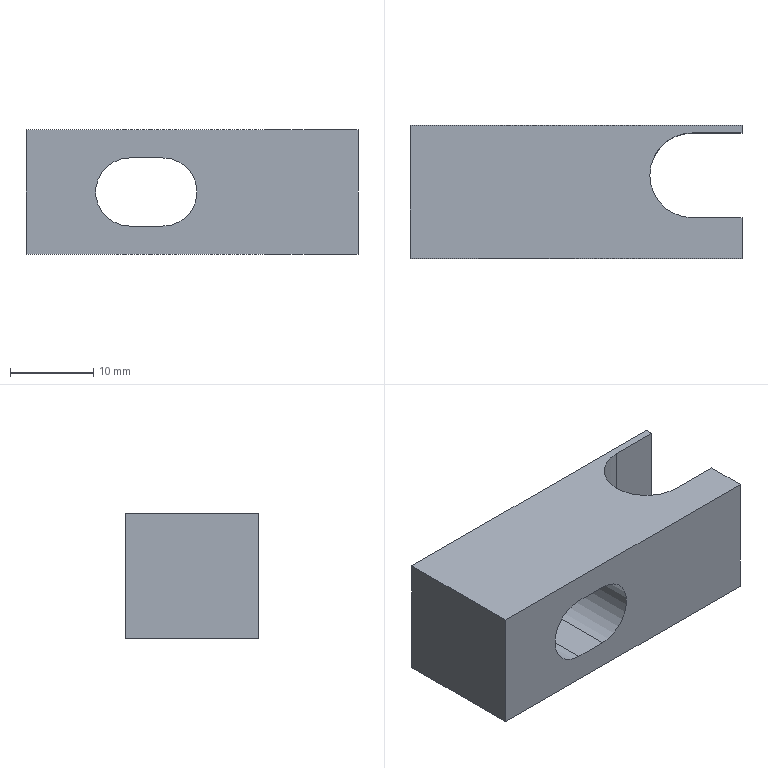Part | STEP file | 1 solid | 15 faces | box 40 x 16 x 15 mm | volume 6699 mm3 | plane 11 | cylinder 4 | commonest cylinder face diameters 8.2 x2 10.2 x2
STEP:
#1=CARTESIAN_POINT('',(0.,0.,0.));
#2=DIRECTION('',(0.,0.,1.));
#3=DIRECTION('',(1.,0.,0.));
#4=AXIS2_PLACEMENT_3D('',#1,#2,#3);
#5=CARTESIAN_POINT('',(9.9,2.077,15.));
#6=VERTEX_POINT('',#5);
#7=CARTESIAN_POINT('',(9.9,2.077,0.));
#8=VERTEX_POINT('',#7);
#9=CARTESIAN_POINT('',(9.9,2.077,15.));
#10=DIRECTION('',(0.,0.,-1.));
#11=VECTOR('',#10,1.);
#12=LINE('',#9,#11);
#13=CARTESIAN_POINT('',(9.9,-3.023,15.));
#14=DIRECTION('',(0.,0.,-1.));
#15=DIRECTION('',(-1.,0.,0.));
#16=AXIS2_PLACEMENT_3D('',#13,#14,#15);
#17=CYLINDRICAL_SURFACE('',#16,5.1);
#18=CARTESIAN_POINT('',(1.571,0.));
#19=DIRECTION('',(0.,1.));
#20=VECTOR('',#19,1.);
#21=LINE('',#18,#20);
#22=(GEOMETRIC_REPRESENTATION_CONTEXT(2)PARAMETRIC_REPRESENTATION_CONTEXT()REPRESENTATION_CONTEXT('',''));
#23=DEFINITIONAL_REPRESENTATION('',(#21),#22);
#24=PCURVE('',#17,#23);
#25=CARTESIAN_POINT('',(9.9,2.077,15.));
#26=DIRECTION('',(0.,1.,0.));
#27=DIRECTION('',(0.,0.,1.));
#28=AXIS2_PLACEMENT_3D('',#25,#26,#27);
#29=PLANE('',#28);
#30=CARTESIAN_POINT('',(0.,0.));
#31=DIRECTION('',(-1.,0.));
#32=VECTOR('',#31,1.);
#33=LINE('',#30,#32);
#34=(GEOMETRIC_REPRESENTATION_CONTEXT(2)PARAMETRIC_REPRESENTATION_CONTEXT()REPRESENTATION_CONTEXT('',''));
#35=DEFINITIONAL_REPRESENTATION('',(#33),#34);
#36=PCURVE('',#29,#35);
#37=SURFACE_CURVE('',#12,(#24,#36),.PCURVE_S1.);
#38=EDGE_CURVE('',#6,#8,#37,.T.);
#39=ORIENTED_EDGE('',*,*,#38,.T.);
#40=CARTESIAN_POINT('',(4.8,-3.023,0.));
#41=VERTEX_POINT('',#40);
#42=CARTESIAN_POINT('',(9.9,-3.023,0.));
#43=DIRECTION('',(0.,0.,-1.));
#44=DIRECTION('',(1.,0.,0.));
#45=AXIS2_PLACEMENT_3D('',#42,#43,#44);
#46=CIRCLE('',#45,5.1);
#47=CARTESIAN_POINT('',(-3.142,15.));
#48=DIRECTION('',(1.,0.));
#49=VECTOR('',#48,1.);
#50=LINE('',#47,#49);
#51=(GEOMETRIC_REPRESENTATION_CONTEXT(2)PARAMETRIC_REPRESENTATION_CONTEXT()REPRESENTATION_CONTEXT('',''));
#52=DEFINITIONAL_REPRESENTATION('',(#50),#51);
#53=PCURVE('',#17,#52);
#54=CARTESIAN_POINT('',(9.9,-3.023,0.));
#55=DIRECTION('',(0.,0.,1.));
#56=DIRECTION('',(1.,0.,0.));
#57=AXIS2_PLACEMENT_3D('',#54,#55,#56);
#58=PLANE('',#57);
#59=CARTESIAN_POINT('',(5.1,0.));
#60=CARTESIAN_POINT('',(5.1,-8.833));
#61=CARTESIAN_POINT('',(-2.55,-4.417));
#62=CARTESIAN_POINT('',(-10.2,0.));
#63=CARTESIAN_POINT('',(-2.55,4.417));
#64=CARTESIAN_POINT('',(5.1,8.833));
#65=CARTESIAN_POINT('',(5.1,0.));
#66=(BOUNDED_CURVE()B_SPLINE_CURVE(2,(#59,#60,#61,#62,#63,#64,#65),.UNSPECIFIED.,.T.,.F.)B_SPLINE_CURVE_WITH_KNOTS((1,2,2,2,2,1),(-2.094,0.,2.094,4.189,6.283,8.378),.UNSPECIFIED.)CURVE()GEOMETRIC_REPRESENTATION_ITEM()RATIONAL_B_SPLINE_CURVE((1.,0.5,1.,0.5,1.,0.5,1.))REPRESENTATION_ITEM(''));
#67=(GEOMETRIC_REPRESENTATION_CONTEXT(2)PARAMETRIC_REPRESENTATION_CONTEXT()REPRESENTATION_CONTEXT('',''));
#68=DEFINITIONAL_REPRESENTATION('',(#66),#67);
#69=PCURVE('',#58,#68);
#70=SURFACE_CURVE('',#46,(#53,#69),.PCURVE_S1.);
#71=EDGE_CURVE('',#41,#8,#70,.T.);
#72=ORIENTED_EDGE('',*,*,#71,.F.);
#73=CARTESIAN_POINT('',(4.8,-3.023,15.));
#74=VERTEX_POINT('',#73);
#75=CARTESIAN_POINT('',(4.8,-3.023,15.));
#76=DIRECTION('',(0.,0.,-1.));
#77=VECTOR('',#76,1.);
#78=LINE('',#75,#77);
#79=CARTESIAN_POINT('',(0.,0.));
#80=DIRECTION('',(0.,1.));
#81=VECTOR('',#80,1.);
#82=LINE('',#79,#81);
#83=(GEOMETRIC_REPRESENTATION_CONTEXT(2)PARAMETRIC_REPRESENTATION_CONTEXT()REPRESENTATION_CONTEXT('',''));
#84=DEFINITIONAL_REPRESENTATION('',(#82),#83);
#85=PCURVE('',#17,#84);
#86=CARTESIAN_POINT('',(9.9,-3.023,15.));
#87=DIRECTION('',(0.,0.,-1.));
#88=DIRECTION('',(-1.,0.,0.));
#89=AXIS2_PLACEMENT_3D('',#86,#87,#88);
#90=CYLINDRICAL_SURFACE('',#89,5.1);
#91=CARTESIAN_POINT('',(6.283,0.));
#92=DIRECTION('',(0.,1.));
#93=VECTOR('',#92,1.);
#94=LINE('',#91,#93);
#95=(GEOMETRIC_REPRESENTATION_CONTEXT(2)PARAMETRIC_REPRESENTATION_CONTEXT()REPRESENTATION_CONTEXT('',''));
#96=DEFINITIONAL_REPRESENTATION('',(#94),#95);
#97=PCURVE('',#90,#96);
#98=SURFACE_CURVE('',#78,(#85,#97),.PCURVE_S1.);
#99=EDGE_CURVE('',#74,#41,#98,.T.);
#100=ORIENTED_EDGE('',*,*,#99,.F.);
#101=CARTESIAN_POINT('',(9.9,-3.023,15.));
#102=DIRECTION('',(0.,0.,-1.));
#103=DIRECTION('',(1.,0.,0.));
#104=AXIS2_PLACEMENT_3D('',#101,#102,#103);
#105=CIRCLE('',#104,5.1);
#106=CARTESIAN_POINT('',(-3.142,0.));
#107=DIRECTION('',(1.,0.));
#108=VECTOR('',#107,1.);
#109=LINE('',#106,#108);
#110=(GEOMETRIC_REPRESENTATION_CONTEXT(2)PARAMETRIC_REPRESENTATION_CONTEXT()REPRESENTATION_CONTEXT('',''));
#111=DEFINITIONAL_REPRESENTATION('',(#109),#110);
#112=PCURVE('',#17,#111);
#113=CARTESIAN_POINT('',(9.9,-3.023,15.));
#114=DIRECTION('',(0.,0.,1.));
#115=DIRECTION('',(1.,0.,0.));
#116=AXIS2_PLACEMENT_3D('',#113,#114,#115);
#117=PLANE('',#116);
#118=CARTESIAN_POINT('',(5.1,0.));
#119=CARTESIAN_POINT('',(5.1,-8.833));
#120=CARTESIAN_POINT('',(-2.55,-4.417));
#121=CARTESIAN_POINT('',(-10.2,0.));
#122=CARTESIAN_POINT('',(-2.55,4.417));
#123=CARTESIAN_POINT('',(5.1,8.833));
#124=CARTESIAN_POINT('',(5.1,0.));
#125=(BOUNDED_CURVE()B_SPLINE_CURVE(2,(#118,#119,#120,#121,#122,#123,#124),.UNSPECIFIED.,.T.,.F.)B_SPLINE_CURVE_WITH_KNOTS((1,2,2,2,2,1),(-2.094,0.,2.094,4.189,6.283,8.378),.UNSPECIFIED.)CURVE()GEOMETRIC_REPRESENTATION_ITEM()RATIONAL_B_SPLINE_CURVE((1.,0.5,1.,0.5,1.,0.5,1.))REPRESENTATION_ITEM(''));
#126=(GEOMETRIC_REPRESENTATION_CONTEXT(2)PARAMETRIC_REPRESENTATION_CONTEXT()REPRESENTATION_CONTEXT('',''));
#127=DEFINITIONAL_REPRESENTATION('',(#125),#126);
#128=PCURVE('',#117,#127);
#129=SURFACE_CURVE('',#105,(#112,#128),.PCURVE_S1.);
#130=EDGE_CURVE('',#74,#6,#129,.T.);
#131=ORIENTED_EDGE('',*,*,#130,.T.);
#132=EDGE_LOOP('',(#39,#72,#100,#131));
#133=FACE_BOUND('',#132,.F.);
#134=ADVANCED_FACE('',(#133),#17,.F.);
#135=CARTESIAN_POINT('',(9.9,-8.123,0.));
#136=VERTEX_POINT('',#135);
#137=CARTESIAN_POINT('',(9.9,-3.023,0.));
#138=DIRECTION('',(0.,0.,-1.));
#139=DIRECTION('',(1.,0.,0.));
#140=AXIS2_PLACEMENT_3D('',#137,#138,#139);
#141=CIRCLE('',#140,5.1);
#142=CARTESIAN_POINT('',(3.142,15.));
#143=DIRECTION('',(1.,0.));
#144=VECTOR('',#143,1.);
#145=LINE('',#142,#144);
#146=(GEOMETRIC_REPRESENTATION_CONTEXT(2)PARAMETRIC_REPRESENTATION_CONTEXT()REPRESENTATION_CONTEXT('',''));
#147=DEFINITIONAL_REPRESENTATION('',(#145),#146);
#148=PCURVE('',#90,#147);
#149=CARTESIAN_POINT('',(5.1,0.));
#150=CARTESIAN_POINT('',(5.1,-8.833));
#151=CARTESIAN_POINT('',(-2.55,-4.417));
#152=CARTESIAN_POINT('',(-10.2,0.));
#153=CARTESIAN_POINT('',(-2.55,4.417));
#154=CARTESIAN_POINT('',(5.1,8.833));
#155=CARTESIAN_POINT('',(5.1,0.));
#156=(BOUNDED_CURVE()B_SPLINE_CURVE(2,(#149,#150,#151,#152,#153,#154,#155),.UNSPECIFIED.,.T.,.F.)B_SPLINE_CURVE_WITH_KNOTS((1,2,2,2,2,1),(-2.094,0.,2.094,4.189,6.283,8.378),.UNSPECIFIED.)CURVE()GEOMETRIC_REPRESENTATION_ITEM()RATIONAL_B_SPLINE_CURVE((1.,0.5,1.,0.5,1.,0.5,1.))REPRESENTATION_ITEM(''));
#157=(GEOMETRIC_REPRESENTATION_CONTEXT(2)PARAMETRIC_REPRESENTATION_CONTEXT()REPRESENTATION_CONTEXT('',''));
#158=DEFINITIONAL_REPRESENTATION('',(#156),#157);
#159=PCURVE('',#58,#158);
#160=SURFACE_CURVE('',#141,(#148,#159),.PCURVE_S1.);
#161=EDGE_CURVE('',#136,#41,#160,.T.);
#162=ORIENTED_EDGE('',*,*,#161,.F.);
#163=CARTESIAN_POINT('',(9.9,-8.123,15.));
#164=VERTEX_POINT('',#163);
#165=CARTESIAN_POINT('',(9.9,-8.123,15.));
#166=DIRECTION('',(0.,0.,-1.));
#167=VECTOR('',#166,1.);
#168=LINE('',#165,#167);
#169=CARTESIAN_POINT('',(4.712,0.));
#170=DIRECTION('',(0.,1.));
#171=VECTOR('',#170,1.);
#172=LINE('',#169,#171);
#173=(GEOMETRIC_REPRESENTATION_CONTEXT(2)PARAMETRIC_REPRESENTATION_CONTEXT()REPRESENTATION_CONTEXT('',''));
#174=DEFINITIONAL_REPRESENTATION('',(#172),#173);
#175=PCURVE('',#90,#174);
#176=CARTESIAN_POINT('',(9.9,-8.123,15.));
#177=DIRECTION('',(0.,-1.,0.));
#178=DIRECTION('',(0.,0.,-1.));
#179=AXIS2_PLACEMENT_3D('',#176,#177,#178);
#180=PLANE('',#179);
#181=CARTESIAN_POINT('',(0.,0.));
#182=DIRECTION('',(1.,0.));
#183=VECTOR('',#182,1.);
#184=LINE('',#181,#183);
#185=(GEOMETRIC_REPRESENTATION_CONTEXT(2)PARAMETRIC_REPRESENTATION_CONTEXT()REPRESENTATION_CONTEXT('',''));
#186=DEFINITIONAL_REPRESENTATION('',(#184),#185);
#187=PCURVE('',#180,#186);
#188=SURFACE_CURVE('',#168,(#175,#187),.PCURVE_S1.);
#189=EDGE_CURVE('',#164,#136,#188,.T.);
#190=ORIENTED_EDGE('',*,*,#189,.F.);
#191=CARTESIAN_POINT('',(9.9,-3.023,15.));
#192=DIRECTION('',(0.,0.,-1.));
#193=DIRECTION('',(1.,0.,0.));
#194=AXIS2_PLACEMENT_3D('',#191,#192,#193);
#195=CIRCLE('',#194,5.1);
#196=CARTESIAN_POINT('',(3.142,0.));
#197=DIRECTION('',(1.,0.));
#198=VECTOR('',#197,1.);
#199=LINE('',#196,#198);
#200=(GEOMETRIC_REPRESENTATION_CONTEXT(2)PARAMETRIC_REPRESENTATION_CONTEXT()REPRESENTATION_CONTEXT('',''));
#201=DEFINITIONAL_REPRESENTATION('',(#199),#200);
#202=PCURVE('',#90,#201);
#203=CARTESIAN_POINT('',(5.1,0.));
#204=CARTESIAN_POINT('',(5.1,-8.833));
#205=CARTESIAN_POINT('',(-2.55,-4.417));
#206=CARTESIAN_POINT('',(-10.2,0.));
#207=CARTESIAN_POINT('',(-2.55,4.417));
#208=CARTESIAN_POINT('',(5.1,8.833));
#209=CARTESIAN_POINT('',(5.1,0.));
#210=(BOUNDED_CURVE()B_SPLINE_CURVE(2,(#203,#204,#205,#206,#207,#208,#209),.UNSPECIFIED.,.T.,.F.)B_SPLINE_CURVE_WITH_KNOTS((1,2,2,2,2,1),(-2.094,0.,2.094,4.189,6.283,8.378),.UNSPECIFIED.)CURVE()GEOMETRIC_REPRESENTATION_ITEM()RATIONAL_B_SPLINE_CURVE((1.,0.5,1.,0.5,1.,0.5,1.))REPRESENTATION_ITEM(''));
#211=(GEOMETRIC_REPRESENTATION_CONTEXT(2)PARAMETRIC_REPRESENTATION_CONTEXT()REPRESENTATION_CONTEXT('',''));
#212=DEFINITIONAL_REPRESENTATION('',(#210),#211);
#213=PCURVE('',#117,#212);
#214=SURFACE_CURVE('',#195,(#202,#213),.PCURVE_S1.);
#215=EDGE_CURVE('',#164,#74,#214,.T.);
#216=ORIENTED_EDGE('',*,*,#215,.T.);
#217=ORIENTED_EDGE('',*,*,#99,.T.);
#218=EDGE_LOOP('',(#162,#190,#216,#217));
#219=FACE_BOUND('',#218,.F.);
#220=ADVANCED_FACE('',(#219),#90,.F.);
#221=CARTESIAN_POINT('',(15.9,2.077,0.));
#222=VERTEX_POINT('',#221);
#223=CARTESIAN_POINT('',(9.9,2.077,0.));
#224=DIRECTION('',(1.,0.,0.));
#225=VECTOR('',#224,1.);
#226=LINE('',#223,#225);
#227=CARTESIAN_POINT('',(-15.,0.));
#228=DIRECTION('',(0.,1.));
#229=VECTOR('',#228,1.);
#230=LINE('',#227,#229);
#231=(GEOMETRIC_REPRESENTATION_CONTEXT(2)PARAMETRIC_REPRESENTATION_CONTEXT()REPRESENTATION_CONTEXT('',''));
#232=DEFINITIONAL_REPRESENTATION('',(#230),#231);
#233=PCURVE('',#29,#232);
#234=CARTESIAN_POINT('',(0.,5.1));
#235=DIRECTION('',(1.,0.));
#236=VECTOR('',#235,1.);
#237=LINE('',#234,#236);
#238=(GEOMETRIC_REPRESENTATION_CONTEXT(2)PARAMETRIC_REPRESENTATION_CONTEXT()REPRESENTATION_CONTEXT('',''));
#239=DEFINITIONAL_REPRESENTATION('',(#237),#238);
#240=PCURVE('',#58,#239);
#241=SURFACE_CURVE('',#226,(#233,#240),.PCURVE_S1.);
#242=EDGE_CURVE('',#8,#222,#241,.T.);
#243=ORIENTED_EDGE('',*,*,#242,.T.);
#244=CARTESIAN_POINT('',(15.9,2.077,15.));
#245=VERTEX_POINT('',#244);
#246=CARTESIAN_POINT('',(15.9,2.077,15.));
#247=DIRECTION('',(0.,0.,-1.));
#248=VECTOR('',#247,1.);
#249=LINE('',#246,#248);
#250=CARTESIAN_POINT('',(0.,6.));
#251=DIRECTION('',(-1.,0.));
#252=VECTOR('',#251,1.);
#253=LINE('',#250,#252);
#254=(GEOMETRIC_REPRESENTATION_CONTEXT(2)PARAMETRIC_REPRESENTATION_CONTEXT()REPRESENTATION_CONTEXT('',''));
#255=DEFINITIONAL_REPRESENTATION('',(#253),#254);
#256=PCURVE('',#29,#255);
#257=CARTESIAN_POINT('',(15.9,2.977,15.));
#258=DIRECTION('',(-1.,0.,0.));
#259=DIRECTION('',(0.,0.,1.));
#260=AXIS2_PLACEMENT_3D('',#257,#258,#259);
#261=PLANE('',#260);
#262=CARTESIAN_POINT('',(0.,-0.9));
#263=DIRECTION('',(-1.,0.));
#264=VECTOR('',#263,1.);
#265=LINE('',#262,#264);
#266=(GEOMETRIC_REPRESENTATION_CONTEXT(2)PARAMETRIC_REPRESENTATION_CONTEXT()REPRESENTATION_CONTEXT('',''));
#267=DEFINITIONAL_REPRESENTATION('',(#265),#266);
#268=PCURVE('',#261,#267);
#269=SURFACE_CURVE('',#249,(#256,#268),.PCURVE_S1.);
#270=EDGE_CURVE('',#245,#222,#269,.T.);
#271=ORIENTED_EDGE('',*,*,#270,.F.);
#272=CARTESIAN_POINT('',(9.9,2.077,15.));
#273=DIRECTION('',(1.,0.,0.));
#274=VECTOR('',#273,1.);
#275=LINE('',#272,#274);
#276=CARTESIAN_POINT('',(0.,0.));
#277=DIRECTION('',(0.,1.));
#278=VECTOR('',#277,1.);
#279=LINE('',#276,#278);
#280=(GEOMETRIC_REPRESENTATION_CONTEXT(2)PARAMETRIC_REPRESENTATION_CONTEXT()REPRESENTATION_CONTEXT('',''));
#281=DEFINITIONAL_REPRESENTATION('',(#279),#280);
#282=PCURVE('',#29,#281);
#283=CARTESIAN_POINT('',(0.,5.1));
#284=DIRECTION('',(1.,0.));
#285=VECTOR('',#284,1.);
#286=LINE('',#283,#285);
#287=(GEOMETRIC_REPRESENTATION_CONTEXT(2)PARAMETRIC_REPRESENTATION_CONTEXT()REPRESENTATION_CONTEXT('',''));
#288=DEFINITIONAL_REPRESENTATION('',(#286),#287);
#289=PCURVE('',#117,#288);
#290=SURFACE_CURVE('',#275,(#282,#289),.PCURVE_S1.);
#291=EDGE_CURVE('',#6,#245,#290,.T.);
#292=ORIENTED_EDGE('',*,*,#291,.F.);
#293=ORIENTED_EDGE('',*,*,#38,.T.);
#294=EDGE_LOOP('',(#243,#271,#292,#293));
#295=FACE_BOUND('',#294,.T.);
#296=ADVANCED_FACE('',(#295),#29,.F.);
#297=CARTESIAN_POINT('',(15.9,2.977,0.));
#298=VERTEX_POINT('',#297);
#299=CARTESIAN_POINT('',(15.9,2.977,0.));
#300=DIRECTION('',(0.,1.,0.));
#301=VECTOR('',#300,1.);
#302=LINE('',#299,#301);
#303=CARTESIAN_POINT('',(-15.,0.));
#304=DIRECTION('',(0.,1.));
#305=VECTOR('',#304,1.);
#306=LINE('',#303,#305);
#307=(GEOMETRIC_REPRESENTATION_CONTEXT(2)PARAMETRIC_REPRESENTATION_CONTEXT()REPRESENTATION_CONTEXT('',''));
#308=DEFINITIONAL_REPRESENTATION('',(#306),#307);
#309=PCURVE('',#261,#308);
#310=CARTESIAN_POINT('',(6.,6.));
#311=DIRECTION('',(0.,1.));
#312=VECTOR('',#311,1.);
#313=LINE('',#310,#312);
#314=(GEOMETRIC_REPRESENTATION_CONTEXT(2)PARAMETRIC_REPRESENTATION_CONTEXT()REPRESENTATION_CONTEXT('',''));
#315=DEFINITIONAL_REPRESENTATION('',(#313),#314);
#316=PCURVE('',#58,#315);
#317=SURFACE_CURVE('',#302,(#309,#316),.PCURVE_S1.);
#318=EDGE_CURVE('',#222,#298,#317,.T.);
#319=ORIENTED_EDGE('',*,*,#318,.T.);
#320=CARTESIAN_POINT('',(15.9,2.977,15.));
#321=VERTEX_POINT('',#320);
#322=CARTESIAN_POINT('',(15.9,2.977,15.));
#323=DIRECTION('',(0.,0.,-1.));
#324=VECTOR('',#323,1.);
#325=LINE('',#322,#324);
#326=CARTESIAN_POINT('',(0.,0.));
#327=DIRECTION('',(-1.,0.));
#328=VECTOR('',#327,1.);
#329=LINE('',#326,#328);
#330=(GEOMETRIC_REPRESENTATION_CONTEXT(2)PARAMETRIC_REPRESENTATION_CONTEXT()REPRESENTATION_CONTEXT('',''));
#331=DEFINITIONAL_REPRESENTATION('',(#329),#330);
#332=PCURVE('',#261,#331);
#333=CARTESIAN_POINT('',(-24.1,2.977,15.));
#334=DIRECTION('',(0.,-1.,0.));
#335=DIRECTION('',(1.,0.,0.));
#336=AXIS2_PLACEMENT_3D('',#333,#334,#335);
#337=PLANE('',#336);
#338=CARTESIAN_POINT('',(40.,0.));
#339=DIRECTION('',(0.,-1.));
#340=VECTOR('',#339,1.);
#341=LINE('',#338,#340);
#342=(GEOMETRIC_REPRESENTATION_CONTEXT(2)PARAMETRIC_REPRESENTATION_CONTEXT()REPRESENTATION_CONTEXT('',''));
#343=DEFINITIONAL_REPRESENTATION('',(#341),#342);
#344=PCURVE('',#337,#343);
#345=SURFACE_CURVE('',#325,(#332,#344),.PCURVE_S1.);
#346=EDGE_CURVE('',#321,#298,#345,.T.);
#347=ORIENTED_EDGE('',*,*,#346,.F.);
#348=CARTESIAN_POINT('',(15.9,2.977,15.));
#349=DIRECTION('',(0.,1.,0.));
#350=VECTOR('',#349,1.);
#351=LINE('',#348,#350);
#352=CARTESIAN_POINT('',(0.,0.));
#353=DIRECTION('',(0.,1.));
#354=VECTOR('',#353,1.);
#355=LINE('',#352,#354);
#356=(GEOMETRIC_REPRESENTATION_CONTEXT(2)PARAMETRIC_REPRESENTATION_CONTEXT()REPRESENTATION_CONTEXT('',''));
#357=DEFINITIONAL_REPRESENTATION('',(#355),#356);
#358=PCURVE('',#261,#357);
#359=CARTESIAN_POINT('',(6.,6.));
#360=DIRECTION('',(0.,1.));
#361=VECTOR('',#360,1.);
#362=LINE('',#359,#361);
#363=(GEOMETRIC_REPRESENTATION_CONTEXT(2)PARAMETRIC_REPRESENTATION_CONTEXT()REPRESENTATION_CONTEXT('',''));
#364=DEFINITIONAL_REPRESENTATION('',(#362),#363);
#365=PCURVE('',#117,#364);
#366=SURFACE_CURVE('',#351,(#358,#365),.PCURVE_S1.);
#367=EDGE_CURVE('',#245,#321,#366,.T.);
#368=ORIENTED_EDGE('',*,*,#367,.F.);
#369=ORIENTED_EDGE('',*,*,#270,.T.);
#370=EDGE_LOOP('',(#319,#347,#368,#369));
#371=FACE_BOUND('',#370,.T.);
#372=ADVANCED_FACE('',(#371),#261,.F.);
#373=CARTESIAN_POINT('',(-11.6,2.977,3.4));
#374=VERTEX_POINT('',#373);
#375=CARTESIAN_POINT('',(-7.6,2.977,3.4));
#376=VERTEX_POINT('',#375);
#377=CARTESIAN_POINT('',(-7.6,2.977,3.4));
#378=DIRECTION('',(1.,0.,0.));
#379=VECTOR('',#378,1.);
#380=LINE('',#377,#379);
#381=CARTESIAN_POINT('',(16.5,-11.6));
#382=DIRECTION('',(1.,0.));
#383=VECTOR('',#382,1.);
#384=LINE('',#381,#383);
#385=(GEOMETRIC_REPRESENTATION_CONTEXT(2)PARAMETRIC_REPRESENTATION_CONTEXT()REPRESENTATION_CONTEXT('',''));
#386=DEFINITIONAL_REPRESENTATION('',(#384),#385);
#387=PCURVE('',#337,#386);
#388=CARTESIAN_POINT('',(-7.6,2.977,3.4));
#389=DIRECTION('',(0.,0.,-1.));
#390=DIRECTION('',(-1.,0.,0.));
#391=AXIS2_PLACEMENT_3D('',#388,#389,#390);
#392=PLANE('',#391);
#393=CARTESIAN_POINT('',(0.,0.));
#394=DIRECTION('',(-1.,0.));
#395=VECTOR('',#394,1.);
#396=LINE('',#393,#395);
#397=(GEOMETRIC_REPRESENTATION_CONTEXT(2)PARAMETRIC_REPRESENTATION_CONTEXT()REPRESENTATION_CONTEXT('',''));
#398=DEFINITIONAL_REPRESENTATION('',(#396),#397);
#399=PCURVE('',#392,#398);
#400=SURFACE_CURVE('',#380,(#387,#399),.PCURVE_S1.);
#401=EDGE_CURVE('',#374,#376,#400,.T.);
#402=ORIENTED_EDGE('',*,*,#401,.T.);
#403=CARTESIAN_POINT('',(-7.6,2.977,11.6));
#404=VERTEX_POINT('',#403);
#405=CARTESIAN_POINT('',(-7.6,2.977,7.5));
#406=DIRECTION('',(0.,-1.,0.));
#407=DIRECTION('',(0.,0.,-1.));
#408=AXIS2_PLACEMENT_3D('',#405,#406,#407);
#409=CIRCLE('',#408,4.1);
#410=CARTESIAN_POINT('',(16.5,-7.5));
#411=DIRECTION('',(0.,-1.));
#412=AXIS2_PLACEMENT_2D('',#410,#411);
#413=CIRCLE('',#412,4.1);
#414=(GEOMETRIC_REPRESENTATION_CONTEXT(2)PARAMETRIC_REPRESENTATION_CONTEXT()REPRESENTATION_CONTEXT('',''));
#415=DEFINITIONAL_REPRESENTATION('',(#413),#414);
#416=PCURVE('',#337,#415);
#417=CARTESIAN_POINT('',(-7.6,2.977,7.5));
#418=DIRECTION('',(0.,-1.,0.));
#419=DIRECTION('',(0.,0.,-1.));
#420=AXIS2_PLACEMENT_3D('',#417,#418,#419);
#421=CYLINDRICAL_SURFACE('',#420,4.1);
#422=CARTESIAN_POINT('',(0.,0.));
#423=DIRECTION('',(1.,0.));
#424=VECTOR('',#423,1.);
#425=LINE('',#422,#424);
#426=(GEOMETRIC_REPRESENTATION_CONTEXT(2)PARAMETRIC_REPRESENTATION_CONTEXT()REPRESENTATION_CONTEXT('',''));
#427=DEFINITIONAL_REPRESENTATION('',(#425),#426);
#428=PCURVE('',#421,#427);
#429=SURFACE_CURVE('',#409,(#416,#428),.PCURVE_S1.);
#430=EDGE_CURVE('',#376,#404,#429,.T.);
#431=ORIENTED_EDGE('',*,*,#430,.T.);
#432=CARTESIAN_POINT('',(-11.6,2.977,11.6));
#433=VERTEX_POINT('',#432);
#434=CARTESIAN_POINT('',(-7.6,2.977,11.6));
#435=DIRECTION('',(-1.,0.,0.));
#436=VECTOR('',#435,1.);
#437=LINE('',#434,#436);
#438=CARTESIAN_POINT('',(16.5,-3.4));
#439=DIRECTION('',(-1.,0.));
#440=VECTOR('',#439,1.);
#441=LINE('',#438,#440);
#442=(GEOMETRIC_REPRESENTATION_CONTEXT(2)PARAMETRIC_REPRESENTATION_CONTEXT()REPRESENTATION_CONTEXT('',''));
#443=DEFINITIONAL_REPRESENTATION('',(#441),#442);
#444=PCURVE('',#337,#443);
#445=CARTESIAN_POINT('',(-7.6,2.977,11.6));
#446=DIRECTION('',(0.,0.,1.));
#447=DIRECTION('',(1.,0.,0.));
#448=AXIS2_PLACEMENT_3D('',#445,#446,#447);
#449=PLANE('',#448);
#450=CARTESIAN_POINT('',(0.,0.));
#451=DIRECTION('',(-1.,0.));
#452=VECTOR('',#451,1.);
#453=LINE('',#450,#452);
#454=(GEOMETRIC_REPRESENTATION_CONTEXT(2)PARAMETRIC_REPRESENTATION_CONTEXT()REPRESENTATION_CONTEXT('',''));
#455=DEFINITIONAL_REPRESENTATION('',(#453),#454);
#456=PCURVE('',#449,#455);
#457=SURFACE_CURVE('',#437,(#444,#456),.PCURVE_S1.);
#458=EDGE_CURVE('',#404,#433,#457,.T.);
#459=ORIENTED_EDGE('',*,*,#458,.T.);
#460=CARTESIAN_POINT('',(-11.6,2.977,7.5));
#461=DIRECTION('',(0.,-1.,0.));
#462=DIRECTION('',(0.,0.,-1.));
#463=AXIS2_PLACEMENT_3D('',#460,#461,#462);
#464=CIRCLE('',#463,4.1);
#465=CARTESIAN_POINT('',(12.5,-7.5));
#466=DIRECTION('',(0.,-1.));
#467=AXIS2_PLACEMENT_2D('',#465,#466);
#468=CIRCLE('',#467,4.1);
#469=(GEOMETRIC_REPRESENTATION_CONTEXT(2)PARAMETRIC_REPRESENTATION_CONTEXT()REPRESENTATION_CONTEXT('',''));
#470=DEFINITIONAL_REPRESENTATION('',(#468),#469);
#471=PCURVE('',#337,#470);
#472=CARTESIAN_POINT('',(-11.6,2.977,7.5));
#473=DIRECTION('',(0.,-1.,0.));
#474=DIRECTION('',(0.,0.,-1.));
#475=AXIS2_PLACEMENT_3D('',#472,#473,#474);
#476=CYLINDRICAL_SURFACE('',#475,4.1);
#477=CARTESIAN_POINT('',(0.,0.));
#478=DIRECTION('',(1.,0.));
#479=VECTOR('',#478,1.);
#480=LINE('',#477,#479);
#481=(GEOMETRIC_REPRESENTATION_CONTEXT(2)PARAMETRIC_REPRESENTATION_CONTEXT()REPRESENTATION_CONTEXT('',''));
#482=DEFINITIONAL_REPRESENTATION('',(#480),#481);
#483=PCURVE('',#476,#482);
#484=SURFACE_CURVE('',#464,(#471,#483),.PCURVE_S1.);
#485=EDGE_CURVE('',#433,#374,#484,.T.);
#486=ORIENTED_EDGE('',*,*,#485,.T.);
#487=EDGE_LOOP('',(#402,#431,#459,#486));
#488=FACE_BOUND('',#487,.T.);
#489=CARTESIAN_POINT('',(-24.1,2.977,0.));
#490=VERTEX_POINT('',#489);
#491=CARTESIAN_POINT('',(-24.1,2.977,0.));
#492=DIRECTION('',(-1.,0.,0.));
#493=VECTOR('',#492,1.);
#494=LINE('',#491,#493);
#495=CARTESIAN_POINT('',(0.,-15.));
#496=DIRECTION('',(-1.,0.));
#497=VECTOR('',#496,1.);
#498=LINE('',#495,#497);
#499=(GEOMETRIC_REPRESENTATION_CONTEXT(2)PARAMETRIC_REPRESENTATION_CONTEXT()REPRESENTATION_CONTEXT('',''));
#500=DEFINITIONAL_REPRESENTATION('',(#498),#499);
#501=PCURVE('',#337,#500);
#502=CARTESIAN_POINT('',(-34.,6.));
#503=DIRECTION('',(-1.,0.));
#504=VECTOR('',#503,1.);
#505=LINE('',#502,#504);
#506=(GEOMETRIC_REPRESENTATION_CONTEXT(2)PARAMETRIC_REPRESENTATION_CONTEXT()REPRESENTATION_CONTEXT('',''));
#507=DEFINITIONAL_REPRESENTATION('',(#505),#506);
#508=PCURVE('',#58,#507);
#509=SURFACE_CURVE('',#494,(#501,#508),.PCURVE_S1.);
#510=EDGE_CURVE('',#298,#490,#509,.T.);
#511=ORIENTED_EDGE('',*,*,#510,.T.);
#512=CARTESIAN_POINT('',(-24.1,2.977,15.));
#513=VERTEX_POINT('',#512);
#514=CARTESIAN_POINT('',(-24.1,2.977,15.));
#515=DIRECTION('',(0.,0.,-1.));
#516=VECTOR('',#515,1.);
#517=LINE('',#514,#516);
#518=CARTESIAN_POINT('',(0.,0.));
#519=DIRECTION('',(0.,-1.));
#520=VECTOR('',#519,1.);
#521=LINE('',#518,#520);
#522=(GEOMETRIC_REPRESENTATION_CONTEXT(2)PARAMETRIC_REPRESENTATION_CONTEXT()REPRESENTATION_CONTEXT('',''));
#523=DEFINITIONAL_REPRESENTATION('',(#521),#522);
#524=PCURVE('',#337,#523);
#525=CARTESIAN_POINT('',(-24.1,2.977,15.));
#526=DIRECTION('',(1.,0.,0.));
#527=DIRECTION('',(0.,0.,-1.));
#528=AXIS2_PLACEMENT_3D('',#525,#526,#527);
#529=PLANE('',#528);
#530=CARTESIAN_POINT('',(0.,0.));
#531=DIRECTION('',(1.,0.));
#532=VECTOR('',#531,1.);
#533=LINE('',#530,#532);
#534=(GEOMETRIC_REPRESENTATION_CONTEXT(2)PARAMETRIC_REPRESENTATION_CONTEXT()REPRESENTATION_CONTEXT('',''));
#535=DEFINITIONAL_REPRESENTATION('',(#533),#534);
#536=PCURVE('',#529,#535);
#537=SURFACE_CURVE('',#517,(#524,#536),.PCURVE_S1.);
#538=EDGE_CURVE('',#513,#490,#537,.T.);
#539=ORIENTED_EDGE('',*,*,#538,.F.);
#540=CARTESIAN_POINT('',(-24.1,2.977,15.));
#541=DIRECTION('',(-1.,0.,0.));
#542=VECTOR('',#541,1.);
#543=LINE('',#540,#542);
#544=CARTESIAN_POINT('',(0.,0.));
#545=DIRECTION('',(-1.,0.));
#546=VECTOR('',#545,1.);
#547=LINE('',#544,#546);
#548=(GEOMETRIC_REPRESENTATION_CONTEXT(2)PARAMETRIC_REPRESENTATION_CONTEXT()REPRESENTATION_CONTEXT('',''));
#549=DEFINITIONAL_REPRESENTATION('',(#547),#548);
#550=PCURVE('',#337,#549);
#551=CARTESIAN_POINT('',(-34.,6.));
#552=DIRECTION('',(-1.,0.));
#553=VECTOR('',#552,1.);
#554=LINE('',#551,#553);
#555=(GEOMETRIC_REPRESENTATION_CONTEXT(2)PARAMETRIC_REPRESENTATION_CONTEXT()REPRESENTATION_CONTEXT('',''));
#556=DEFINITIONAL_REPRESENTATION('',(#554),#555);
#557=PCURVE('',#117,#556);
#558=SURFACE_CURVE('',#543,(#550,#557),.PCURVE_S1.);
#559=EDGE_CURVE('',#321,#513,#558,.T.);
#560=ORIENTED_EDGE('',*,*,#559,.F.);
#561=ORIENTED_EDGE('',*,*,#346,.T.);
#562=EDGE_LOOP('',(#511,#539,#560,#561));
#563=FACE_BOUND('',#562,.T.);
#564=ADVANCED_FACE('',(#488,#563),#337,.F.);
#565=CARTESIAN_POINT('',(-24.1,-13.023,0.));
#566=VERTEX_POINT('',#565);
#567=CARTESIAN_POINT('',(-24.1,2.977,0.));
#568=DIRECTION('',(0.,-1.,0.));
#569=VECTOR('',#568,1.);
#570=LINE('',#567,#569);
#571=CARTESIAN_POINT('',(15.,0.));
#572=DIRECTION('',(0.,-1.));
#573=VECTOR('',#572,1.);
#574=LINE('',#571,#573);
#575=(GEOMETRIC_REPRESENTATION_CONTEXT(2)PARAMETRIC_REPRESENTATION_CONTEXT()REPRESENTATION_CONTEXT('',''));
#576=DEFINITIONAL_REPRESENTATION('',(#574),#575);
#577=PCURVE('',#529,#576);
#578=CARTESIAN_POINT('',(-34.,6.));
#579=DIRECTION('',(0.,-1.));
#580=VECTOR('',#579,1.);
#581=LINE('',#578,#580);
#582=(GEOMETRIC_REPRESENTATION_CONTEXT(2)PARAMETRIC_REPRESENTATION_CONTEXT()REPRESENTATION_CONTEXT('',''));
#583=DEFINITIONAL_REPRESENTATION('',(#581),#582);
#584=PCURVE('',#58,#583);
#585=SURFACE_CURVE('',#570,(#577,#584),.PCURVE_S1.);
#586=EDGE_CURVE('',#490,#566,#585,.T.);
#587=ORIENTED_EDGE('',*,*,#586,.T.);
#588=CARTESIAN_POINT('',(-24.1,-13.023,15.));
#589=VERTEX_POINT('',#588);
#590=CARTESIAN_POINT('',(-24.1,-13.023,15.));
#591=DIRECTION('',(0.,0.,-1.));
#592=VECTOR('',#591,1.);
#593=LINE('',#590,#592);
#594=CARTESIAN_POINT('',(0.,-16.));
#595=DIRECTION('',(1.,0.));
#596=VECTOR('',#595,1.);
#597=LINE('',#594,#596);
#598=(GEOMETRIC_REPRESENTATION_CONTEXT(2)PARAMETRIC_REPRESENTATION_CONTEXT()REPRESENTATION_CONTEXT('',''));
#599=DEFINITIONAL_REPRESENTATION('',(#597),#598);
#600=PCURVE('',#529,#599);
#601=CARTESIAN_POINT('',(-24.1,-13.023,15.));
#602=DIRECTION('',(0.,1.,0.));
#603=DIRECTION('',(0.,0.,1.));
#604=AXIS2_PLACEMENT_3D('',#601,#602,#603);
#605=PLANE('',#604);
#606=CARTESIAN_POINT('',(0.,0.));
#607=DIRECTION('',(-1.,0.));
#608=VECTOR('',#607,1.);
#609=LINE('',#606,#608);
#610=(GEOMETRIC_REPRESENTATION_CONTEXT(2)PARAMETRIC_REPRESENTATION_CONTEXT()REPRESENTATION_CONTEXT('',''));
#611=DEFINITIONAL_REPRESENTATION('',(#609),#610);
#612=PCURVE('',#605,#611);
#613=SURFACE_CURVE('',#593,(#600,#612),.PCURVE_S1.);
#614=EDGE_CURVE('',#589,#566,#613,.T.);
#615=ORIENTED_EDGE('',*,*,#614,.F.);
#616=CARTESIAN_POINT('',(-24.1,2.977,15.));
#617=DIRECTION('',(0.,-1.,0.));
#618=VECTOR('',#617,1.);
#619=LINE('',#616,#618);
#620=CARTESIAN_POINT('',(0.,0.));
#621=DIRECTION('',(0.,-1.));
#622=VECTOR('',#621,1.);
#623=LINE('',#620,#622);
#624=(GEOMETRIC_REPRESENTATION_CONTEXT(2)PARAMETRIC_REPRESENTATION_CONTEXT()REPRESENTATION_CONTEXT('',''));
#625=DEFINITIONAL_REPRESENTATION('',(#623),#624);
#626=PCURVE('',#529,#625);
#627=CARTESIAN_POINT('',(-34.,6.));
#628=DIRECTION('',(0.,-1.));
#629=VECTOR('',#628,1.);
#630=LINE('',#627,#629);
#631=(GEOMETRIC_REPRESENTATION_CONTEXT(2)PARAMETRIC_REPRESENTATION_CONTEXT()REPRESENTATION_CONTEXT('',''));
#632=DEFINITIONAL_REPRESENTATION('',(#630),#631);
#633=PCURVE('',#117,#632);
#634=SURFACE_CURVE('',#619,(#626,#633),.PCURVE_S1.);
#635=EDGE_CURVE('',#513,#589,#634,.T.);
#636=ORIENTED_EDGE('',*,*,#635,.F.);
#637=ORIENTED_EDGE('',*,*,#538,.T.);
#638=EDGE_LOOP('',(#587,#615,#636,#637));
#639=FACE_BOUND('',#638,.T.);
#640=ADVANCED_FACE('',(#639),#529,.F.);
#641=CARTESIAN_POINT('',(-7.6,-13.023,11.6));
#642=VERTEX_POINT('',#641);
#643=CARTESIAN_POINT('',(-11.6,-13.023,11.6));
#644=VERTEX_POINT('',#643);
#645=CARTESIAN_POINT('',(-7.6,-13.023,11.6));
#646=DIRECTION('',(-1.,0.,0.));
#647=VECTOR('',#646,1.);
#648=LINE('',#645,#647);
#649=CARTESIAN_POINT('',(-3.4,16.5));
#650=DIRECTION('',(0.,-1.));
#651=VECTOR('',#650,1.);
#652=LINE('',#649,#651);
#653=(GEOMETRIC_REPRESENTATION_CONTEXT(2)PARAMETRIC_REPRESENTATION_CONTEXT()REPRESENTATION_CONTEXT('',''));
#654=DEFINITIONAL_REPRESENTATION('',(#652),#653);
#655=PCURVE('',#605,#654);
#656=CARTESIAN_POINT('',(0.,-16.));
#657=DIRECTION('',(-1.,0.));
#658=VECTOR('',#657,1.);
#659=LINE('',#656,#658);
#660=(GEOMETRIC_REPRESENTATION_CONTEXT(2)PARAMETRIC_REPRESENTATION_CONTEXT()REPRESENTATION_CONTEXT('',''));
#661=DEFINITIONAL_REPRESENTATION('',(#659),#660);
#662=PCURVE('',#449,#661);
#663=SURFACE_CURVE('',#648,(#655,#662),.PCURVE_S1.);
#664=EDGE_CURVE('',#642,#644,#663,.T.);
#665=ORIENTED_EDGE('',*,*,#664,.F.);
#666=CARTESIAN_POINT('',(-7.6,-13.023,3.4));
#667=VERTEX_POINT('',#666);
#668=CARTESIAN_POINT('',(-7.6,-13.023,7.5));
#669=DIRECTION('',(0.,-1.,0.));
#670=DIRECTION('',(0.,0.,-1.));
#671=AXIS2_PLACEMENT_3D('',#668,#669,#670);
#672=CIRCLE('',#671,4.1);
#673=CARTESIAN_POINT('',(-11.6,16.5));
#674=CARTESIAN_POINT('',(-11.6,23.601));
#675=CARTESIAN_POINT('',(-5.45,20.051));
#676=CARTESIAN_POINT('',(0.7,16.5));
#677=CARTESIAN_POINT('',(-5.45,12.949));
#678=CARTESIAN_POINT('',(-11.6,9.399));
#679=CARTESIAN_POINT('',(-11.6,16.5));
#680=(BOUNDED_CURVE()B_SPLINE_CURVE(2,(#673,#674,#675,#676,#677,#678,#679),.UNSPECIFIED.,.T.,.F.)B_SPLINE_CURVE_WITH_KNOTS((1,2,2,2,2,1),(-2.094,0.,2.094,4.189,6.283,8.378),.UNSPECIFIED.)CURVE()GEOMETRIC_REPRESENTATION_ITEM()RATIONAL_B_SPLINE_CURVE((1.,0.5,1.,0.5,1.,0.5,1.))REPRESENTATION_ITEM(''));
#681=(GEOMETRIC_REPRESENTATION_CONTEXT(2)PARAMETRIC_REPRESENTATION_CONTEXT()REPRESENTATION_CONTEXT('',''));
#682=DEFINITIONAL_REPRESENTATION('',(#680),#681);
#683=PCURVE('',#605,#682);
#684=CARTESIAN_POINT('',(0.,16.));
#685=DIRECTION('',(1.,0.));
#686=VECTOR('',#685,1.);
#687=LINE('',#684,#686);
#688=(GEOMETRIC_REPRESENTATION_CONTEXT(2)PARAMETRIC_REPRESENTATION_CONTEXT()REPRESENTATION_CONTEXT('',''));
#689=DEFINITIONAL_REPRESENTATION('',(#687),#688);
#690=PCURVE('',#421,#689);
#691=SURFACE_CURVE('',#672,(#683,#690),.PCURVE_S1.);
#692=EDGE_CURVE('',#667,#642,#691,.T.);
#693=ORIENTED_EDGE('',*,*,#692,.F.);
#694=CARTESIAN_POINT('',(-11.6,-13.023,3.4));
#695=VERTEX_POINT('',#694);
#696=CARTESIAN_POINT('',(-7.6,-13.023,3.4));
#697=DIRECTION('',(1.,0.,0.));
#698=VECTOR('',#697,1.);
#699=LINE('',#696,#698);
#700=CARTESIAN_POINT('',(-11.6,16.5));
#701=DIRECTION('',(0.,1.));
#702=VECTOR('',#701,1.);
#703=LINE('',#700,#702);
#704=(GEOMETRIC_REPRESENTATION_CONTEXT(2)PARAMETRIC_REPRESENTATION_CONTEXT()REPRESENTATION_CONTEXT('',''));
#705=DEFINITIONAL_REPRESENTATION('',(#703),#704);
#706=PCURVE('',#605,#705);
#707=CARTESIAN_POINT('',(0.,-16.));
#708=DIRECTION('',(-1.,0.));
#709=VECTOR('',#708,1.);
#710=LINE('',#707,#709);
#711=(GEOMETRIC_REPRESENTATION_CONTEXT(2)PARAMETRIC_REPRESENTATION_CONTEXT()REPRESENTATION_CONTEXT('',''));
#712=DEFINITIONAL_REPRESENTATION('',(#710),#711);
#713=PCURVE('',#392,#712);
#714=SURFACE_CURVE('',#699,(#706,#713),.PCURVE_S1.);
#715=EDGE_CURVE('',#695,#667,#714,.T.);
#716=ORIENTED_EDGE('',*,*,#715,.F.);
#717=CARTESIAN_POINT('',(-11.6,-13.023,7.5));
#718=DIRECTION('',(0.,-1.,0.));
#719=DIRECTION('',(0.,0.,-1.));
#720=AXIS2_PLACEMENT_3D('',#717,#718,#719);
#721=CIRCLE('',#720,4.1);
#722=CARTESIAN_POINT('',(-11.6,12.5));
#723=CARTESIAN_POINT('',(-11.6,19.601));
#724=CARTESIAN_POINT('',(-5.45,16.051));
#725=CARTESIAN_POINT('',(0.7,12.5));
#726=CARTESIAN_POINT('',(-5.45,8.949));
#727=CARTESIAN_POINT('',(-11.6,5.399));
#728=CARTESIAN_POINT('',(-11.6,12.5));
#729=(BOUNDED_CURVE()B_SPLINE_CURVE(2,(#722,#723,#724,#725,#726,#727,#728),.UNSPECIFIED.,.T.,.F.)B_SPLINE_CURVE_WITH_KNOTS((1,2,2,2,2,1),(-2.094,0.,2.094,4.189,6.283,8.378),.UNSPECIFIED.)CURVE()GEOMETRIC_REPRESENTATION_ITEM()RATIONAL_B_SPLINE_CURVE((1.,0.5,1.,0.5,1.,0.5,1.))REPRESENTATION_ITEM(''));
#730=(GEOMETRIC_REPRESENTATION_CONTEXT(2)PARAMETRIC_REPRESENTATION_CONTEXT()REPRESENTATION_CONTEXT('',''));
#731=DEFINITIONAL_REPRESENTATION('',(#729),#730);
#732=PCURVE('',#605,#731);
#733=CARTESIAN_POINT('',(0.,16.));
#734=DIRECTION('',(1.,0.));
#735=VECTOR('',#734,1.);
#736=LINE('',#733,#735);
#737=(GEOMETRIC_REPRESENTATION_CONTEXT(2)PARAMETRIC_REPRESENTATION_CONTEXT()REPRESENTATION_CONTEXT('',''));
#738=DEFINITIONAL_REPRESENTATION('',(#736),#737);
#739=PCURVE('',#476,#738);
#740=SURFACE_CURVE('',#721,(#732,#739),.PCURVE_S1.);
#741=EDGE_CURVE('',#644,#695,#740,.T.);
#742=ORIENTED_EDGE('',*,*,#741,.F.);
#743=EDGE_LOOP('',(#665,#693,#716,#742));
#744=FACE_BOUND('',#743,.T.);
#745=CARTESIAN_POINT('',(15.9,-13.023,0.));
#746=VERTEX_POINT('',#745);
#747=CARTESIAN_POINT('',(-24.1,-13.023,0.));
#748=DIRECTION('',(1.,0.,0.));
#749=VECTOR('',#748,1.);
#750=LINE('',#747,#749);
#751=CARTESIAN_POINT('',(-15.,0.));
#752=DIRECTION('',(0.,1.));
#753=VECTOR('',#752,1.);
#754=LINE('',#751,#753);
#755=(GEOMETRIC_REPRESENTATION_CONTEXT(2)PARAMETRIC_REPRESENTATION_CONTEXT()REPRESENTATION_CONTEXT('',''));
#756=DEFINITIONAL_REPRESENTATION('',(#754),#755);
#757=PCURVE('',#605,#756);
#758=CARTESIAN_POINT('',(-34.,-10.));
#759=DIRECTION('',(1.,0.));
#760=VECTOR('',#759,1.);
#761=LINE('',#758,#760);
#762=(GEOMETRIC_REPRESENTATION_CONTEXT(2)PARAMETRIC_REPRESENTATION_CONTEXT()REPRESENTATION_CONTEXT('',''));
#763=DEFINITIONAL_REPRESENTATION('',(#761),#762);
#764=PCURVE('',#58,#763);
#765=SURFACE_CURVE('',#750,(#757,#764),.PCURVE_S1.);
#766=EDGE_CURVE('',#566,#746,#765,.T.);
#767=ORIENTED_EDGE('',*,*,#766,.T.);
#768=CARTESIAN_POINT('',(15.9,-13.023,15.));
#769=VERTEX_POINT('',#768);
#770=CARTESIAN_POINT('',(15.9,-13.023,15.));
#771=DIRECTION('',(0.,0.,-1.));
#772=VECTOR('',#771,1.);
#773=LINE('',#770,#772);
#774=CARTESIAN_POINT('',(0.,40.));
#775=DIRECTION('',(-1.,0.));
#776=VECTOR('',#775,1.);
#777=LINE('',#774,#776);
#778=(GEOMETRIC_REPRESENTATION_CONTEXT(2)PARAMETRIC_REPRESENTATION_CONTEXT()REPRESENTATION_CONTEXT('',''));
#779=DEFINITIONAL_REPRESENTATION('',(#777),#778);
#780=PCURVE('',#605,#779);
#781=CARTESIAN_POINT('',(15.9,-8.123,15.));
#782=DIRECTION('',(-1.,0.,0.));
#783=DIRECTION('',(0.,0.,1.));
#784=AXIS2_PLACEMENT_3D('',#781,#782,#783);
#785=PLANE('',#784);
#786=CARTESIAN_POINT('',(0.,-4.9));
#787=DIRECTION('',(-1.,0.));
#788=VECTOR('',#787,1.);
#789=LINE('',#786,#788);
#790=(GEOMETRIC_REPRESENTATION_CONTEXT(2)PARAMETRIC_REPRESENTATION_CONTEXT()REPRESENTATION_CONTEXT('',''));
#791=DEFINITIONAL_REPRESENTATION('',(#789),#790);
#792=PCURVE('',#785,#791);
#793=SURFACE_CURVE('',#773,(#780,#792),.PCURVE_S1.);
#794=EDGE_CURVE('',#769,#746,#793,.T.);
#795=ORIENTED_EDGE('',*,*,#794,.F.);
#796=CARTESIAN_POINT('',(-24.1,-13.023,15.));
#797=DIRECTION('',(1.,0.,0.));
#798=VECTOR('',#797,1.);
#799=LINE('',#796,#798);
#800=CARTESIAN_POINT('',(0.,0.));
#801=DIRECTION('',(0.,1.));
#802=VECTOR('',#801,1.);
#803=LINE('',#800,#802);
#804=(GEOMETRIC_REPRESENTATION_CONTEXT(2)PARAMETRIC_REPRESENTATION_CONTEXT()REPRESENTATION_CONTEXT('',''));
#805=DEFINITIONAL_REPRESENTATION('',(#803),#804);
#806=PCURVE('',#605,#805);
#807=CARTESIAN_POINT('',(-34.,-10.));
#808=DIRECTION('',(1.,0.));
#809=VECTOR('',#808,1.);
#810=LINE('',#807,#809);
#811=(GEOMETRIC_REPRESENTATION_CONTEXT(2)PARAMETRIC_REPRESENTATION_CONTEXT()REPRESENTATION_CONTEXT('',''));
#812=DEFINITIONAL_REPRESENTATION('',(#810),#811);
#813=PCURVE('',#117,#812);
#814=SURFACE_CURVE('',#799,(#806,#813),.PCURVE_S1.);
#815=EDGE_CURVE('',#589,#769,#814,.T.);
#816=ORIENTED_EDGE('',*,*,#815,.F.);
#817=ORIENTED_EDGE('',*,*,#614,.T.);
#818=EDGE_LOOP('',(#767,#795,#816,#817));
#819=FACE_BOUND('',#818,.T.);
#820=ADVANCED_FACE('',(#744,#819),#605,.F.);
#821=CARTESIAN_POINT('',(15.9,-8.123,0.));
#822=VERTEX_POINT('',#821);
#823=CARTESIAN_POINT('',(15.9,-8.123,0.));
#824=DIRECTION('',(0.,1.,0.));
#825=VECTOR('',#824,1.);
#826=LINE('',#823,#825);
#827=CARTESIAN_POINT('',(-15.,0.));
#828=DIRECTION('',(0.,1.));
#829=VECTOR('',#828,1.);
#830=LINE('',#827,#829);
#831=(GEOMETRIC_REPRESENTATION_CONTEXT(2)PARAMETRIC_REPRESENTATION_CONTEXT()REPRESENTATION_CONTEXT('',''));
#832=DEFINITIONAL_REPRESENTATION('',(#830),#831);
#833=PCURVE('',#785,#832);
#834=CARTESIAN_POINT('',(6.,-5.1));
#835=DIRECTION('',(0.,1.));
#836=VECTOR('',#835,1.);
#837=LINE('',#834,#836);
#838=(GEOMETRIC_REPRESENTATION_CONTEXT(2)PARAMETRIC_REPRESENTATION_CONTEXT()REPRESENTATION_CONTEXT('',''));
#839=DEFINITIONAL_REPRESENTATION('',(#837),#838);
#840=PCURVE('',#58,#839);
#841=SURFACE_CURVE('',#826,(#833,#840),.PCURVE_S1.);
#842=EDGE_CURVE('',#746,#822,#841,.T.);
#843=ORIENTED_EDGE('',*,*,#842,.T.);
#844=CARTESIAN_POINT('',(15.9,-8.123,15.));
#845=VERTEX_POINT('',#844);
#846=CARTESIAN_POINT('',(15.9,-8.123,15.));
#847=DIRECTION('',(0.,0.,-1.));
#848=VECTOR('',#847,1.);
#849=LINE('',#846,#848);
#850=CARTESIAN_POINT('',(0.,0.));
#851=DIRECTION('',(-1.,0.));
#852=VECTOR('',#851,1.);
#853=LINE('',#850,#852);
#854=(GEOMETRIC_REPRESENTATION_CONTEXT(2)PARAMETRIC_REPRESENTATION_CONTEXT()REPRESENTATION_CONTEXT('',''));
#855=DEFINITIONAL_REPRESENTATION('',(#853),#854);
#856=PCURVE('',#785,#855);
#857=CARTESIAN_POINT('',(0.,6.));
#858=DIRECTION('',(1.,0.));
#859=VECTOR('',#858,1.);
#860=LINE('',#857,#859);
#861=(GEOMETRIC_REPRESENTATION_CONTEXT(2)PARAMETRIC_REPRESENTATION_CONTEXT()REPRESENTATION_CONTEXT('',''));
#862=DEFINITIONAL_REPRESENTATION('',(#860),#861);
#863=PCURVE('',#180,#862);
#864=SURFACE_CURVE('',#849,(#856,#863),.PCURVE_S1.);
#865=EDGE_CURVE('',#845,#822,#864,.T.);
#866=ORIENTED_EDGE('',*,*,#865,.F.);
#867=CARTESIAN_POINT('',(15.9,-8.123,15.));
#868=DIRECTION('',(0.,1.,0.));
#869=VECTOR('',#868,1.);
#870=LINE('',#867,#869);
#871=CARTESIAN_POINT('',(0.,0.));
#872=DIRECTION('',(0.,1.));
#873=VECTOR('',#872,1.);
#874=LINE('',#871,#873);
#875=(GEOMETRIC_REPRESENTATION_CONTEXT(2)PARAMETRIC_REPRESENTATION_CONTEXT()REPRESENTATION_CONTEXT('',''));
#876=DEFINITIONAL_REPRESENTATION('',(#874),#875);
#877=PCURVE('',#785,#876);
#878=CARTESIAN_POINT('',(6.,-5.1));
#879=DIRECTION('',(0.,1.));
#880=VECTOR('',#879,1.);
#881=LINE('',#878,#880);
#882=(GEOMETRIC_REPRESENTATION_CONTEXT(2)PARAMETRIC_REPRESENTATION_CONTEXT()REPRESENTATION_CONTEXT('',''));
#883=DEFINITIONAL_REPRESENTATION('',(#881),#882);
#884=PCURVE('',#117,#883);
#885=SURFACE_CURVE('',#870,(#877,#884),.PCURVE_S1.);
#886=EDGE_CURVE('',#769,#845,#885,.T.);
#887=ORIENTED_EDGE('',*,*,#886,.F.);
#888=ORIENTED_EDGE('',*,*,#794,.T.);
#889=EDGE_LOOP('',(#843,#866,#887,#888));
#890=FACE_BOUND('',#889,.T.);
#891=ADVANCED_FACE('',(#890),#785,.F.);
#892=CARTESIAN_POINT('',(9.9,-8.123,0.));
#893=DIRECTION('',(-1.,0.,0.));
#894=VECTOR('',#893,1.);
#895=LINE('',#892,#894);
#896=CARTESIAN_POINT('',(15.,0.));
#897=DIRECTION('',(0.,-1.));
#898=VECTOR('',#897,1.);
#899=LINE('',#896,#898);
#900=(GEOMETRIC_REPRESENTATION_CONTEXT(2)PARAMETRIC_REPRESENTATION_CONTEXT()REPRESENTATION_CONTEXT('',''));
#901=DEFINITIONAL_REPRESENTATION('',(#899),#900);
#902=PCURVE('',#180,#901);
#903=CARTESIAN_POINT('',(0.,-5.1));
#904=DIRECTION('',(-1.,0.));
#905=VECTOR('',#904,1.);
#906=LINE('',#903,#905);
#907=(GEOMETRIC_REPRESENTATION_CONTEXT(2)PARAMETRIC_REPRESENTATION_CONTEXT()REPRESENTATION_CONTEXT('',''));
#908=DEFINITIONAL_REPRESENTATION('',(#906),#907);
#909=PCURVE('',#58,#908);
#910=SURFACE_CURVE('',#895,(#902,#909),.PCURVE_S1.);
#911=EDGE_CURVE('',#822,#136,#910,.T.);
#912=ORIENTED_EDGE('',*,*,#911,.T.);
#913=ORIENTED_EDGE('',*,*,#189,.F.);
#914=CARTESIAN_POINT('',(9.9,-8.123,15.));
#915=DIRECTION('',(-1.,0.,0.));
#916=VECTOR('',#915,1.);
#917=LINE('',#914,#916);
#918=CARTESIAN_POINT('',(0.,0.));
#919=DIRECTION('',(0.,-1.));
#920=VECTOR('',#919,1.);
#921=LINE('',#918,#920);
#922=(GEOMETRIC_REPRESENTATION_CONTEXT(2)PARAMETRIC_REPRESENTATION_CONTEXT()REPRESENTATION_CONTEXT('',''));
#923=DEFINITIONAL_REPRESENTATION('',(#921),#922);
#924=PCURVE('',#180,#923);
#925=CARTESIAN_POINT('',(0.,-5.1));
#926=DIRECTION('',(-1.,0.));
#927=VECTOR('',#926,1.);
#928=LINE('',#925,#927);
#929=(GEOMETRIC_REPRESENTATION_CONTEXT(2)PARAMETRIC_REPRESENTATION_CONTEXT()REPRESENTATION_CONTEXT('',''));
#930=DEFINITIONAL_REPRESENTATION('',(#928),#929);
#931=PCURVE('',#117,#930);
#932=SURFACE_CURVE('',#917,(#924,#931),.PCURVE_S1.);
#933=EDGE_CURVE('',#845,#164,#932,.T.);
#934=ORIENTED_EDGE('',*,*,#933,.F.);
#935=ORIENTED_EDGE('',*,*,#865,.T.);
#936=EDGE_LOOP('',(#912,#913,#934,#935));
#937=FACE_BOUND('',#936,.T.);
#938=ADVANCED_FACE('',(#937),#180,.F.);
#939=ORIENTED_EDGE('',*,*,#215,.T.);
#940=ORIENTED_EDGE('',*,*,#130,.T.);
#941=ORIENTED_EDGE('',*,*,#291,.T.);
#942=ORIENTED_EDGE('',*,*,#367,.T.);
#943=ORIENTED_EDGE('',*,*,#559,.T.);
#944=ORIENTED_EDGE('',*,*,#635,.T.);
#945=ORIENTED_EDGE('',*,*,#815,.T.);
#946=ORIENTED_EDGE('',*,*,#886,.T.);
#947=ORIENTED_EDGE('',*,*,#933,.T.);
#948=EDGE_LOOP('',(#939,#940,#941,#942,#943,#944,#945,#946,#947));
#949=FACE_BOUND('',#948,.T.);
#950=ADVANCED_FACE('',(#949),#117,.T.);
#951=ORIENTED_EDGE('',*,*,#161,.F.);
#952=ORIENTED_EDGE('',*,*,#911,.F.);
#953=ORIENTED_EDGE('',*,*,#842,.F.);
#954=ORIENTED_EDGE('',*,*,#766,.F.);
#955=ORIENTED_EDGE('',*,*,#586,.F.);
#956=ORIENTED_EDGE('',*,*,#510,.F.);
#957=ORIENTED_EDGE('',*,*,#318,.F.);
#958=ORIENTED_EDGE('',*,*,#242,.F.);
#959=ORIENTED_EDGE('',*,*,#71,.F.);
#960=EDGE_LOOP('',(#951,#952,#953,#954,#955,#956,#957,#958,#959));
#961=FACE_BOUND('',#960,.T.);
#962=ADVANCED_FACE('',(#961),#58,.F.);
#963=CARTESIAN_POINT('',(-7.6,2.977,3.4));
#964=DIRECTION('',(0.,-1.,0.));
#965=VECTOR('',#964,1.);
#966=LINE('',#963,#965);
#967=CARTESIAN_POINT('',(0.,0.));
#968=DIRECTION('',(0.,1.));
#969=VECTOR('',#968,1.);
#970=LINE('',#967,#969);
#971=(GEOMETRIC_REPRESENTATION_CONTEXT(2)PARAMETRIC_REPRESENTATION_CONTEXT()REPRESENTATION_CONTEXT('',''));
#972=DEFINITIONAL_REPRESENTATION('',(#970),#971);
#973=PCURVE('',#421,#972);
#974=CARTESIAN_POINT('',(0.,0.));
#975=DIRECTION('',(0.,-1.));
#976=VECTOR('',#975,1.);
#977=LINE('',#974,#976);
#978=(GEOMETRIC_REPRESENTATION_CONTEXT(2)PARAMETRIC_REPRESENTATION_CONTEXT()REPRESENTATION_CONTEXT('',''));
#979=DEFINITIONAL_REPRESENTATION('',(#977),#978);
#980=PCURVE('',#392,#979);
#981=SURFACE_CURVE('',#966,(#973,#980),.PCURVE_S1.);
#982=EDGE_CURVE('',#376,#667,#981,.T.);
#983=ORIENTED_EDGE('',*,*,#982,.F.);
#984=ORIENTED_EDGE('',*,*,#430,.T.);
#985=CARTESIAN_POINT('',(-7.6,2.977,11.6));
#986=DIRECTION('',(0.,-1.,0.));
#987=VECTOR('',#986,1.);
#988=LINE('',#985,#987);
#989=CARTESIAN_POINT('',(3.142,0.));
#990=DIRECTION('',(0.,1.));
#991=VECTOR('',#990,1.);
#992=LINE('',#989,#991);
#993=(GEOMETRIC_REPRESENTATION_CONTEXT(2)PARAMETRIC_REPRESENTATION_CONTEXT()REPRESENTATION_CONTEXT('',''));
#994=DEFINITIONAL_REPRESENTATION('',(#992),#993);
#995=PCURVE('',#421,#994);
#996=CARTESIAN_POINT('',(0.,0.));
#997=DIRECTION('',(0.,-1.));
#998=VECTOR('',#997,1.);
#999=LINE('',#996,#998);
#1000=(GEOMETRIC_REPRESENTATION_CONTEXT(2)PARAMETRIC_REPRESENTATION_CONTEXT()REPRESENTATION_CONTEXT('',''));
#1001=DEFINITIONAL_REPRESENTATION('',(#999),#1000);
#1002=PCURVE('',#449,#1001);
#1003=SURFACE_CURVE('',#988,(#995,#1002),.PCURVE_S1.);
#1004=EDGE_CURVE('',#404,#642,#1003,.T.);
#1005=ORIENTED_EDGE('',*,*,#1004,.T.);
#1006=ORIENTED_EDGE('',*,*,#692,.F.);
#1007=EDGE_LOOP('',(#983,#984,#1005,#1006));
#1008=FACE_BOUND('',#1007,.F.);
#1009=ADVANCED_FACE('',(#1008),#421,.F.);
#1010=ORIENTED_EDGE('',*,*,#715,.T.);
#1011=ORIENTED_EDGE('',*,*,#982,.F.);
#1012=ORIENTED_EDGE('',*,*,#401,.F.);
#1013=CARTESIAN_POINT('',(-11.6,2.977,3.4));
#1014=DIRECTION('',(0.,-1.,0.));
#1015=VECTOR('',#1014,1.);
#1016=LINE('',#1013,#1015);
#1017=CARTESIAN_POINT('',(4.,0.));
#1018=DIRECTION('',(0.,-1.));
#1019=VECTOR('',#1018,1.);
#1020=LINE('',#1017,#1019);
#1021=(GEOMETRIC_REPRESENTATION_CONTEXT(2)PARAMETRIC_REPRESENTATION_CONTEXT()REPRESENTATION_CONTEXT('',''));
#1022=DEFINITIONAL_REPRESENTATION('',(#1020),#1021);
#1023=PCURVE('',#392,#1022);
#1024=CARTESIAN_POINT('',(6.283,0.));
#1025=DIRECTION('',(0.,1.));
#1026=VECTOR('',#1025,1.);
#1027=LINE('',#1024,#1026);
#1028=(GEOMETRIC_REPRESENTATION_CONTEXT(2)PARAMETRIC_REPRESENTATION_CONTEXT()REPRESENTATION_CONTEXT('',''));
#1029=DEFINITIONAL_REPRESENTATION('',(#1027),#1028);
#1030=PCURVE('',#476,#1029);
#1031=SURFACE_CURVE('',#1016,(#1023,#1030),.PCURVE_S1.);
#1032=EDGE_CURVE('',#374,#695,#1031,.T.);
#1033=ORIENTED_EDGE('',*,*,#1032,.T.);
#1034=EDGE_LOOP('',(#1010,#1011,#1012,#1033));
#1035=FACE_BOUND('',#1034,.T.);
#1036=ADVANCED_FACE('',(#1035),#392,.F.);
#1037=CARTESIAN_POINT('',(-11.6,2.977,11.6));
#1038=DIRECTION('',(0.,-1.,0.));
#1039=VECTOR('',#1038,1.);
#1040=LINE('',#1037,#1039);
#1041=CARTESIAN_POINT('',(3.142,0.));
#1042=DIRECTION('',(0.,1.));
#1043=VECTOR('',#1042,1.);
#1044=LINE('',#1041,#1043);
#1045=(GEOMETRIC_REPRESENTATION_CONTEXT(2)PARAMETRIC_REPRESENTATION_CONTEXT()REPRESENTATION_CONTEXT('',''));
#1046=DEFINITIONAL_REPRESENTATION('',(#1044),#1045);
#1047=PCURVE('',#476,#1046);
#1048=CARTESIAN_POINT('',(-4.,0.));
#1049=DIRECTION('',(0.,-1.));
#1050=VECTOR('',#1049,1.);
#1051=LINE('',#1048,#1050);
#1052=(GEOMETRIC_REPRESENTATION_CONTEXT(2)PARAMETRIC_REPRESENTATION_CONTEXT()REPRESENTATION_CONTEXT('',''));
#1053=DEFINITIONAL_REPRESENTATION('',(#1051),#1052);
#1054=PCURVE('',#449,#1053);
#1055=SURFACE_CURVE('',#1040,(#1047,#1054),.PCURVE_S1.);
#1056=EDGE_CURVE('',#433,#644,#1055,.T.);
#1057=ORIENTED_EDGE('',*,*,#1056,.F.);
#1058=ORIENTED_EDGE('',*,*,#485,.T.);
#1059=ORIENTED_EDGE('',*,*,#1032,.T.);
#1060=ORIENTED_EDGE('',*,*,#741,.F.);
#1061=EDGE_LOOP('',(#1057,#1058,#1059,#1060));
#1062=FACE_BOUND('',#1061,.F.);
#1063=ADVANCED_FACE('',(#1062),#476,.F.);
#1064=ORIENTED_EDGE('',*,*,#664,.T.);
#1065=ORIENTED_EDGE('',*,*,#1056,.F.);
#1066=ORIENTED_EDGE('',*,*,#458,.F.);
#1067=ORIENTED_EDGE('',*,*,#1004,.T.);
#1068=EDGE_LOOP('',(#1064,#1065,#1066,#1067));
#1069=FACE_BOUND('',#1068,.T.);
#1070=ADVANCED_FACE('',(#1069),#449,.F.);
#1071=CLOSED_SHELL('',(#134,#220,#296,#372,#564,#640,#820,#891,#938,#950,#962,#1009,#1036,#1063,#1070));
#1072=MANIFOLD_SOLID_BREP('',#1071);
#1073=(LENGTH_UNIT()NAMED_UNIT(*)SI_UNIT(.MILLI.,.METRE.));
#1074=UNCERTAINTY_MEASURE_WITH_UNIT(LENGTH_MEASURE(0.0000001),#1073,'','');
#1075=(NAMED_UNIT(*)PLANE_ANGLE_UNIT()SI_UNIT($,.RADIAN.));
#1076=(NAMED_UNIT(*)SI_UNIT($,.STERADIAN.)SOLID_ANGLE_UNIT());
#1077=(GEOMETRIC_REPRESENTATION_CONTEXT(3)GLOBAL_UNCERTAINTY_ASSIGNED_CONTEXT((#1074))GLOBAL_UNIT_ASSIGNED_CONTEXT((#1073,#1075,#1076))REPRESENTATION_CONTEXT('',''));
#1078=ADVANCED_BREP_SHAPE_REPRESENTATION('',(#4,#1072),#1077);